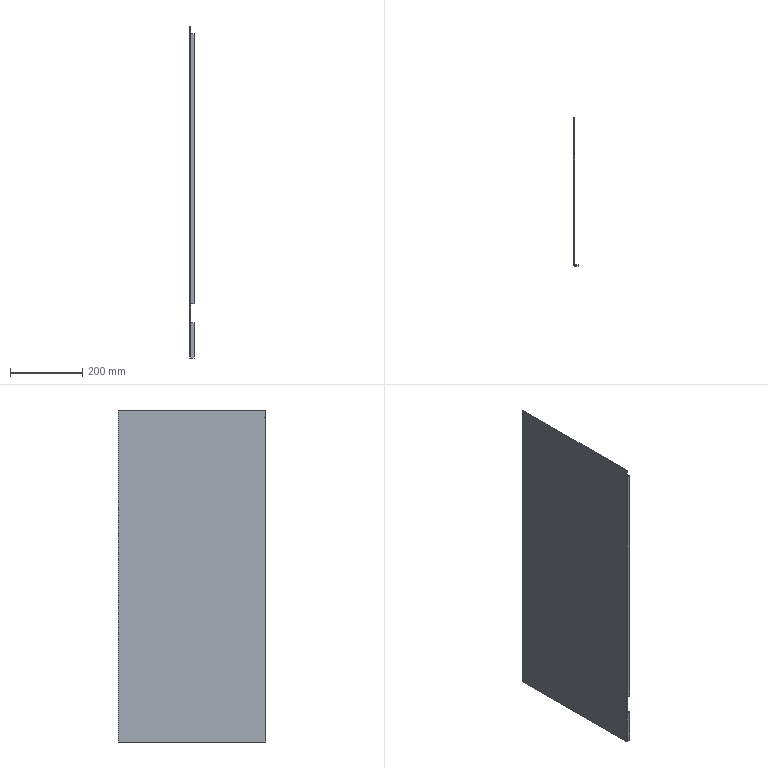Part | SolidWorks | 1 solid | 25 faces | box 12 x 410 x 920 mm | volume 770485 mm3 | plane 23 | cylinder 2 | commonest cylinder face diameters 0.2 x1 4.2 x1
STEP:
#1=CARTESIAN_POINT('',(10.,-205.,-460.));
#2=VERTEX_POINT('',#1);
#3=CARTESIAN_POINT('',(10.,-205.,-362.));
#4=VERTEX_POINT('',#3);
#5=CARTESIAN_POINT('',(10.,-205.,0.));
#6=DIRECTION('',(0.,0.,1.));
#7=VECTOR('',#6,1000.);
#8=LINE('',#5,#7);
#9=EDGE_CURVE('',#2,#4,#8,.T.);
#10=ORIENTED_EDGE('',*,*,#9,.T.);
#11=CARTESIAN_POINT('',(0.1,-205.,-362.));
#12=VERTEX_POINT('',#11);
#13=CARTESIAN_POINT('',(0.,-205.,-362.));
#14=DIRECTION('',(1.,0.,0.));
#15=VECTOR('',#14,1000.);
#16=LINE('',#13,#15);
#17=EDGE_CURVE('',#12,#4,#16,.T.);
#18=ORIENTED_EDGE('',*,*,#17,.F.);
#19=CARTESIAN_POINT('',(0.1,-205.,-460.));
#20=VERTEX_POINT('',#19);
#21=CARTESIAN_POINT('',(0.1,-205.,439.));
#22=DIRECTION('',(0.,0.,1.));
#23=VECTOR('',#22,1000.);
#24=LINE('',#21,#23);
#25=EDGE_CURVE('',#20,#12,#24,.T.);
#26=ORIENTED_EDGE('',*,*,#25,.F.);
#27=CARTESIAN_POINT('',(0.,-205.,-460.));
#28=DIRECTION('',(1.,0.,0.));
#29=VECTOR('',#28,1000.);
#30=LINE('',#27,#29);
#31=EDGE_CURVE('',#20,#2,#30,.T.);
#32=ORIENTED_EDGE('',*,*,#31,.T.);
#33=EDGE_LOOP('',(#10,#18,#26,#32));
#34=FACE_OUTER_BOUND('',#33,.T.);
#35=CARTESIAN_POINT('',(0.,-205.,0.));
#36=DIRECTION('',(0.,1.,0.));
#37=DIRECTION('',(-1.,0.,0.));
#38=AXIS2_PLACEMENT_3D('',#35,#36,#37);
#39=PLANE('',#38);
#40=ADVANCED_FACE('',(#34),#39,.F.);
#41=CARTESIAN_POINT('',(10.,-203.,-362.));
#42=VERTEX_POINT('',#41);
#43=CARTESIAN_POINT('',(0.1,-203.,-362.));
#44=VERTEX_POINT('',#43);
#45=CARTESIAN_POINT('',(0.,-203.,-362.));
#46=DIRECTION('',(-1.,0.,0.));
#47=VECTOR('',#46,1000.);
#48=LINE('',#45,#47);
#49=EDGE_CURVE('',#42,#44,#48,.T.);
#50=ORIENTED_EDGE('',*,*,#49,.F.);
#51=CARTESIAN_POINT('',(10.,-203.,-460.));
#52=VERTEX_POINT('',#51);
#53=CARTESIAN_POINT('',(10.,-203.,439.));
#54=DIRECTION('',(0.,0.,1.));
#55=VECTOR('',#54,1000.);
#56=LINE('',#53,#55);
#57=EDGE_CURVE('',#52,#42,#56,.T.);
#58=ORIENTED_EDGE('',*,*,#57,.F.);
#59=CARTESIAN_POINT('',(0.1,-203.,-460.));
#60=VERTEX_POINT('',#59);
#61=CARTESIAN_POINT('',(10.,-203.,-460.));
#62=DIRECTION('',(1.,0.,0.));
#63=VECTOR('',#62,1000.);
#64=LINE('',#61,#63);
#65=EDGE_CURVE('',#60,#52,#64,.T.);
#66=ORIENTED_EDGE('',*,*,#65,.F.);
#67=CARTESIAN_POINT('',(0.1,-203.,439.));
#68=DIRECTION('',(0.,0.,-1.));
#69=VECTOR('',#68,1000.);
#70=LINE('',#67,#69);
#71=EDGE_CURVE('',#44,#60,#70,.T.);
#72=ORIENTED_EDGE('',*,*,#71,.F.);
#73=EDGE_LOOP('',(#50,#58,#66,#72));
#74=FACE_OUTER_BOUND('',#73,.T.);
#75=CARTESIAN_POINT('',(0.,-203.,0.));
#76=DIRECTION('',(0.,1.,0.));
#77=DIRECTION('',(-1.,0.,0.));
#78=AXIS2_PLACEMENT_3D('',#75,#76,#77);
#79=PLANE('',#78);
#80=ADVANCED_FACE('',(#74),#79,.T.);
#81=ORIENTED_EDGE('',*,*,#57,.T.);
#82=CARTESIAN_POINT('',(10.,-205.001,-362.));
#83=DIRECTION('',(0.,1.,0.));
#84=VECTOR('',#83,1000.);
#85=LINE('',#82,#84);
#86=EDGE_CURVE('',#4,#42,#85,.T.);
#87=ORIENTED_EDGE('',*,*,#86,.F.);
#88=ORIENTED_EDGE('',*,*,#9,.F.);
#89=CARTESIAN_POINT('',(10.,-205.,-460.));
#90=DIRECTION('',(0.,1.,0.));
#91=VECTOR('',#90,1000.);
#92=LINE('',#89,#91);
#93=EDGE_CURVE('',#2,#52,#92,.T.);
#94=ORIENTED_EDGE('',*,*,#93,.T.);
#95=EDGE_LOOP('',(#81,#87,#88,#94));
#96=FACE_OUTER_BOUND('',#95,.T.);
#97=CARTESIAN_POINT('',(10.,-205.,439.));
#98=DIRECTION('',(-1.,0.,0.));
#99=DIRECTION('',(0.,-1.,0.));
#100=AXIS2_PLACEMENT_3D('',#97,#98,#99);
#101=PLANE('',#100);
#102=ADVANCED_FACE('',(#96),#101,.F.);
#103=CARTESIAN_POINT('',(0.,-202.9,-460.));
#104=VERTEX_POINT('',#103);
#105=CARTESIAN_POINT('',(0.,205.,-460.));
#106=VERTEX_POINT('',#105);
#107=CARTESIAN_POINT('',(0.,-205.,-460.));
#108=DIRECTION('',(0.,1.,0.));
#109=VECTOR('',#108,1000.);
#110=LINE('',#107,#109);
#111=EDGE_CURVE('',#104,#106,#110,.T.);
#112=ORIENTED_EDGE('',*,*,#111,.F.);
#113=CARTESIAN_POINT('',(-2.,-202.9,-460.));
#114=VERTEX_POINT('',#113);
#115=CARTESIAN_POINT('',(0.,-202.9,-460.));
#116=DIRECTION('',(-1.,0.,0.));
#117=VECTOR('',#116,1000.);
#118=LINE('',#115,#117);
#119=EDGE_CURVE('',#104,#114,#118,.T.);
#120=ORIENTED_EDGE('',*,*,#119,.T.);
#121=CARTESIAN_POINT('',(-2.,205.,-460.));
#122=VERTEX_POINT('',#121);
#123=CARTESIAN_POINT('',(-2.,-205.,-460.));
#124=DIRECTION('',(0.,1.,0.));
#125=VECTOR('',#124,1000.);
#126=LINE('',#123,#125);
#127=EDGE_CURVE('',#114,#122,#126,.T.);
#128=ORIENTED_EDGE('',*,*,#127,.T.);
#129=CARTESIAN_POINT('',(-2.,205.,-460.));
#130=DIRECTION('',(1.,0.,0.));
#131=VECTOR('',#130,1000.);
#132=LINE('',#129,#131);
#133=EDGE_CURVE('',#122,#106,#132,.T.);
#134=ORIENTED_EDGE('',*,*,#133,.T.);
#135=EDGE_LOOP('',(#112,#120,#128,#134));
#136=FACE_OUTER_BOUND('',#135,.T.);
#137=CARTESIAN_POINT('',(-2.,-205.,-460.));
#138=DIRECTION('',(0.,0.,-1.));
#139=DIRECTION('',(-1.,0.,0.));
#140=AXIS2_PLACEMENT_3D('',#137,#138,#139);
#141=PLANE('',#140);
#142=ADVANCED_FACE('',(#136),#141,.T.);
#143=CARTESIAN_POINT('',(-2.,-205.,460.));
#144=VERTEX_POINT('',#143);
#145=CARTESIAN_POINT('',(-2.,-205.,440.));
#146=VERTEX_POINT('',#145);
#147=CARTESIAN_POINT('',(-2.,-205.,-460.));
#148=DIRECTION('',(0.,0.,-1.));
#149=VECTOR('',#148,1000.);
#150=LINE('',#147,#149);
#151=EDGE_CURVE('',#144,#146,#150,.T.);
#152=ORIENTED_EDGE('',*,*,#151,.T.);
#153=CARTESIAN_POINT('',(0.,-205.,440.));
#154=VERTEX_POINT('',#153);
#155=CARTESIAN_POINT('',(0.,-205.,440.));
#156=DIRECTION('',(-1.,0.,0.));
#157=VECTOR('',#156,1000.);
#158=LINE('',#155,#157);
#159=EDGE_CURVE('',#154,#146,#158,.T.);
#160=ORIENTED_EDGE('',*,*,#159,.F.);
#161=CARTESIAN_POINT('',(0.,-205.,460.));
#162=VERTEX_POINT('',#161);
#163=CARTESIAN_POINT('',(0.,-205.,-460.));
#164=DIRECTION('',(0.,0.,-1.));
#165=VECTOR('',#164,1000.);
#166=LINE('',#163,#165);
#167=EDGE_CURVE('',#162,#154,#166,.T.);
#168=ORIENTED_EDGE('',*,*,#167,.F.);
#169=CARTESIAN_POINT('',(-2.,-205.,460.));
#170=DIRECTION('',(1.,0.,0.));
#171=VECTOR('',#170,1000.);
#172=LINE('',#169,#171);
#173=EDGE_CURVE('',#144,#162,#172,.T.);
#174=ORIENTED_EDGE('',*,*,#173,.F.);
#175=EDGE_LOOP('',(#152,#160,#168,#174));
#176=FACE_OUTER_BOUND('',#175,.T.);
#177=CARTESIAN_POINT('',(-2.,-205.,-460.));
#178=DIRECTION('',(0.,-1.,0.));
#179=DIRECTION('',(0.,0.,-1.));
#180=AXIS2_PLACEMENT_3D('',#177,#178,#179);
#181=PLANE('',#180);
#182=ADVANCED_FACE('',(#176),#181,.T.);
#183=CARTESIAN_POINT('',(-2.,-202.9,439.));
#184=VERTEX_POINT('',#183);
#185=CARTESIAN_POINT('',(-2.,-202.9,-460.));
#186=DIRECTION('',(0.,0.,1.));
#187=VECTOR('',#186,1000.);
#188=LINE('',#185,#187);
#189=EDGE_CURVE('',#114,#184,#188,.T.);
#190=ORIENTED_EDGE('',*,*,#189,.T.);
#191=CARTESIAN_POINT('',(-2.,-201.9,439.));
#192=VERTEX_POINT('',#191);
#193=CARTESIAN_POINT('',(-2.,0.,439.));
#194=DIRECTION('',(0.,-1.,0.));
#195=VECTOR('',#194,1000.);
#196=LINE('',#193,#195);
#197=EDGE_CURVE('',#192,#184,#196,.T.);
#198=ORIENTED_EDGE('',*,*,#197,.F.);
#199=CARTESIAN_POINT('',(-2.,-201.9,440.));
#200=VERTEX_POINT('',#199);
#201=CARTESIAN_POINT('',(-2.,-201.9,0.));
#202=DIRECTION('',(0.,0.,-1.));
#203=VECTOR('',#202,1000.);
#204=LINE('',#201,#203);
#205=EDGE_CURVE('',#200,#192,#204,.T.);
#206=ORIENTED_EDGE('',*,*,#205,.F.);
#207=CARTESIAN_POINT('',(-2.,0.,440.));
#208=DIRECTION('',(0.,1.,0.));
#209=VECTOR('',#208,1000.);
#210=LINE('',#207,#209);
#211=EDGE_CURVE('',#146,#200,#210,.T.);
#212=ORIENTED_EDGE('',*,*,#211,.F.);
#213=ORIENTED_EDGE('',*,*,#151,.F.);
#214=CARTESIAN_POINT('',(-2.,205.,460.));
#215=VERTEX_POINT('',#214);
#216=CARTESIAN_POINT('',(-2.,-205.,460.));
#217=DIRECTION('',(0.,-1.,0.));
#218=VECTOR('',#217,1000.);
#219=LINE('',#216,#218);
#220=EDGE_CURVE('',#215,#144,#219,.T.);
#221=ORIENTED_EDGE('',*,*,#220,.F.);
#222=CARTESIAN_POINT('',(-2.,205.,-460.));
#223=DIRECTION('',(0.,0.,1.));
#224=VECTOR('',#223,1000.);
#225=LINE('',#222,#224);
#226=EDGE_CURVE('',#122,#215,#225,.T.);
#227=ORIENTED_EDGE('',*,*,#226,.F.);
#228=ORIENTED_EDGE('',*,*,#127,.F.);
#229=EDGE_LOOP('',(#190,#198,#206,#212,#213,#221,#227,#228));
#230=FACE_OUTER_BOUND('',#229,.T.);
#231=CARTESIAN_POINT('',(-2.,0.,0.));
#232=DIRECTION('',(1.,0.,0.));
#233=DIRECTION('',(0.,0.,-1.));
#234=AXIS2_PLACEMENT_3D('',#231,#232,#233);
#235=PLANE('',#234);
#236=ADVANCED_FACE('',(#230),#235,.F.);
#237=CARTESIAN_POINT('',(0.,-202.9,439.));
#238=VERTEX_POINT('',#237);
#239=CARTESIAN_POINT('',(0.,-201.9,439.));
#240=VERTEX_POINT('',#239);
#241=CARTESIAN_POINT('',(0.,-202.9,439.));
#242=DIRECTION('',(0.,1.,0.));
#243=VECTOR('',#242,1000.);
#244=LINE('',#241,#243);
#245=EDGE_CURVE('',#238,#240,#244,.T.);
#246=ORIENTED_EDGE('',*,*,#245,.F.);
#247=CARTESIAN_POINT('',(0.,-202.9,-460.));
#248=DIRECTION('',(0.,0.,1.));
#249=VECTOR('',#248,1000.);
#250=LINE('',#247,#249);
#251=EDGE_CURVE('',#104,#238,#250,.T.);
#252=ORIENTED_EDGE('',*,*,#251,.F.);
#253=ORIENTED_EDGE('',*,*,#111,.T.);
#254=CARTESIAN_POINT('',(0.,205.,460.));
#255=VERTEX_POINT('',#254);
#256=CARTESIAN_POINT('',(0.,205.,-460.));
#257=DIRECTION('',(0.,0.,1.));
#258=VECTOR('',#257,1000.);
#259=LINE('',#256,#258);
#260=EDGE_CURVE('',#106,#255,#259,.T.);
#261=ORIENTED_EDGE('',*,*,#260,.T.);
#262=CARTESIAN_POINT('',(0.,-205.,460.));
#263=DIRECTION('',(0.,-1.,0.));
#264=VECTOR('',#263,1000.);
#265=LINE('',#262,#264);
#266=EDGE_CURVE('',#255,#162,#265,.T.);
#267=ORIENTED_EDGE('',*,*,#266,.T.);
#268=ORIENTED_EDGE('',*,*,#167,.T.);
#269=CARTESIAN_POINT('',(0.,-201.9,440.));
#270=VERTEX_POINT('',#269);
#271=CARTESIAN_POINT('',(0.,-201.9,440.));
#272=DIRECTION('',(0.,-1.,0.));
#273=VECTOR('',#272,1000.);
#274=LINE('',#271,#273);
#275=EDGE_CURVE('',#270,#154,#274,.T.);
#276=ORIENTED_EDGE('',*,*,#275,.F.);
#277=CARTESIAN_POINT('',(0.,-201.9,439.));
#278=DIRECTION('',(0.,0.,1.));
#279=VECTOR('',#278,1000.);
#280=LINE('',#277,#279);
#281=EDGE_CURVE('',#240,#270,#280,.T.);
#282=ORIENTED_EDGE('',*,*,#281,.F.);
#283=EDGE_LOOP('',(#246,#252,#253,#261,#267,#268,#276,#282));
#284=FACE_OUTER_BOUND('',#283,.T.);
#285=CARTESIAN_POINT('',(0.,0.,0.));
#286=DIRECTION('',(1.,0.,0.));
#287=DIRECTION('',(0.,0.,-1.));
#288=AXIS2_PLACEMENT_3D('',#285,#286,#287);
#289=PLANE('',#288);
#290=ADVANCED_FACE('',(#284),#289,.T.);
#291=ORIENTED_EDGE('',*,*,#266,.F.);
#292=CARTESIAN_POINT('',(-2.,205.,460.));
#293=DIRECTION('',(1.,0.,0.));
#294=VECTOR('',#293,1000.);
#295=LINE('',#292,#294);
#296=EDGE_CURVE('',#215,#255,#295,.T.);
#297=ORIENTED_EDGE('',*,*,#296,.F.);
#298=ORIENTED_EDGE('',*,*,#220,.T.);
#299=ORIENTED_EDGE('',*,*,#173,.T.);
#300=EDGE_LOOP('',(#291,#297,#298,#299));
#301=FACE_OUTER_BOUND('',#300,.T.);
#302=CARTESIAN_POINT('',(-2.,-205.,460.));
#303=DIRECTION('',(0.,0.,1.));
#304=DIRECTION('',(1.,0.,0.));
#305=AXIS2_PLACEMENT_3D('',#302,#303,#304);
#306=PLANE('',#305);
#307=ADVANCED_FACE('',(#301),#306,.T.);
#308=ORIENTED_EDGE('',*,*,#260,.F.);
#309=ORIENTED_EDGE('',*,*,#133,.F.);
#310=ORIENTED_EDGE('',*,*,#226,.T.);
#311=ORIENTED_EDGE('',*,*,#296,.T.);
#312=EDGE_LOOP('',(#308,#309,#310,#311));
#313=FACE_OUTER_BOUND('',#312,.T.);
#314=CARTESIAN_POINT('',(-2.,205.,-460.));
#315=DIRECTION('',(0.,1.,0.));
#316=DIRECTION('',(0.,0.,1.));
#317=AXIS2_PLACEMENT_3D('',#314,#315,#316);
#318=PLANE('',#317);
#319=ADVANCED_FACE('',(#313),#318,.T.);
#320=CARTESIAN_POINT('',(0.,-201.9,439.));
#321=DIRECTION('',(-1.,0.,0.));
#322=VECTOR('',#321,1000.);
#323=LINE('',#320,#322);
#324=EDGE_CURVE('',#240,#192,#323,.T.);
#325=ORIENTED_EDGE('',*,*,#324,.T.);
#326=ORIENTED_EDGE('',*,*,#197,.T.);
#327=CARTESIAN_POINT('',(0.,-202.9,439.));
#328=DIRECTION('',(-1.,0.,0.));
#329=VECTOR('',#328,1000.);
#330=LINE('',#327,#329);
#331=EDGE_CURVE('',#238,#184,#330,.T.);
#332=ORIENTED_EDGE('',*,*,#331,.F.);
#333=ORIENTED_EDGE('',*,*,#245,.T.);
#334=EDGE_LOOP('',(#325,#326,#332,#333));
#335=FACE_OUTER_BOUND('',#334,.T.);
#336=CARTESIAN_POINT('',(0.,-202.9,439.));
#337=DIRECTION('',(0.,0.,1.));
#338=DIRECTION('',(1.,0.,0.));
#339=AXIS2_PLACEMENT_3D('',#336,#337,#338);
#340=PLANE('',#339);
#341=ADVANCED_FACE('',(#335),#340,.T.);
#342=CARTESIAN_POINT('',(0.,-201.9,440.));
#343=DIRECTION('',(-1.,0.,0.));
#344=VECTOR('',#343,1000.);
#345=LINE('',#342,#344);
#346=EDGE_CURVE('',#270,#200,#345,.T.);
#347=ORIENTED_EDGE('',*,*,#346,.T.);
#348=ORIENTED_EDGE('',*,*,#205,.T.);
#349=ORIENTED_EDGE('',*,*,#324,.F.);
#350=ORIENTED_EDGE('',*,*,#281,.T.);
#351=EDGE_LOOP('',(#347,#348,#349,#350));
#352=FACE_OUTER_BOUND('',#351,.T.);
#353=CARTESIAN_POINT('',(0.,-201.9,439.));
#354=DIRECTION('',(0.,-1.,0.));
#355=DIRECTION('',(0.,0.,-1.));
#356=AXIS2_PLACEMENT_3D('',#353,#354,#355);
#357=PLANE('',#356);
#358=ADVANCED_FACE('',(#352),#357,.T.);
#359=ORIENTED_EDGE('',*,*,#159,.T.);
#360=ORIENTED_EDGE('',*,*,#211,.T.);
#361=ORIENTED_EDGE('',*,*,#346,.F.);
#362=ORIENTED_EDGE('',*,*,#275,.T.);
#363=EDGE_LOOP('',(#359,#360,#361,#362));
#364=FACE_OUTER_BOUND('',#363,.T.);
#365=CARTESIAN_POINT('',(0.,-201.9,440.));
#366=DIRECTION('',(0.,0.,-1.));
#367=DIRECTION('',(-1.,0.,0.));
#368=AXIS2_PLACEMENT_3D('',#365,#366,#367);
#369=PLANE('',#368);
#370=ADVANCED_FACE('',(#364),#369,.T.);
#371=CARTESIAN_POINT('',(0.1,-203.,439.));
#372=VERTEX_POINT('',#371);
#373=CARTESIAN_POINT('',(0.1,-205.,439.));
#374=VERTEX_POINT('',#373);
#375=CARTESIAN_POINT('',(0.1,-205.,439.));
#376=DIRECTION('',(0.,-1.,0.));
#377=VECTOR('',#376,1000.);
#378=LINE('',#375,#377);
#379=EDGE_CURVE('',#372,#374,#378,.T.);
#380=ORIENTED_EDGE('',*,*,#379,.F.);
#381=CARTESIAN_POINT('',(0.1,-202.9,439.));
#382=DIRECTION('',(0.,0.,1.));
#383=DIRECTION('',(-1.,0.,0.));
#384=AXIS2_PLACEMENT_3D('',#381,#382,#383);
#385=CIRCLE('',#384,0.1);
#386=EDGE_CURVE('',#238,#372,#385,.T.);
#387=ORIENTED_EDGE('',*,*,#386,.F.);
#388=ORIENTED_EDGE('',*,*,#331,.T.);
#389=CARTESIAN_POINT('',(0.1,-202.9,439.));
#390=DIRECTION('',(0.,0.,1.));
#391=DIRECTION('',(-1.,0.,0.));
#392=AXIS2_PLACEMENT_3D('',#389,#390,#391);
#393=CIRCLE('',#392,2.1);
#394=EDGE_CURVE('',#184,#374,#393,.T.);
#395=ORIENTED_EDGE('',*,*,#394,.T.);
#396=EDGE_LOOP('',(#380,#387,#388,#395));
#397=FACE_OUTER_BOUND('',#396,.T.);
#398=CARTESIAN_POINT('',(0.1,-202.9,439.));
#399=DIRECTION('',(0.,0.,1.));
#400=DIRECTION('',(1.,0.,0.));
#401=AXIS2_PLACEMENT_3D('',#398,#399,#400);
#402=PLANE('',#401);
#403=ADVANCED_FACE('',(#397),#402,.T.);
#404=CARTESIAN_POINT('',(0.1,-202.9,-460.));
#405=DIRECTION('',(0.,0.,-1.));
#406=DIRECTION('',(-1.,0.,0.));
#407=AXIS2_PLACEMENT_3D('',#404,#405,#406);
#408=CIRCLE('',#407,0.1);
#409=EDGE_CURVE('',#60,#104,#408,.T.);
#410=ORIENTED_EDGE('',*,*,#409,.F.);
#411=CARTESIAN_POINT('',(0.1,-203.,-460.));
#412=DIRECTION('',(0.,-1.,0.));
#413=VECTOR('',#412,1000.);
#414=LINE('',#411,#413);
#415=EDGE_CURVE('',#60,#20,#414,.T.);
#416=ORIENTED_EDGE('',*,*,#415,.T.);
#417=CARTESIAN_POINT('',(0.1,-202.9,-460.));
#418=DIRECTION('',(0.,0.,-1.));
#419=DIRECTION('',(-1.,0.,0.));
#420=AXIS2_PLACEMENT_3D('',#417,#418,#419);
#421=CIRCLE('',#420,2.1);
#422=EDGE_CURVE('',#20,#114,#421,.T.);
#423=ORIENTED_EDGE('',*,*,#422,.T.);
#424=ORIENTED_EDGE('',*,*,#119,.F.);
#425=EDGE_LOOP('',(#410,#416,#423,#424));
#426=FACE_OUTER_BOUND('',#425,.T.);
#427=CARTESIAN_POINT('',(0.1,-202.9,-460.));
#428=DIRECTION('',(0.,0.,1.));
#429=DIRECTION('',(1.,0.,0.));
#430=AXIS2_PLACEMENT_3D('',#427,#428,#429);
#431=PLANE('',#430);
#432=ADVANCED_FACE('',(#426),#431,.F.);
#433=CARTESIAN_POINT('',(0.,-204.998,-362.));
#434=VERTEX_POINT('',#433);
#435=CARTESIAN_POINT('',(0.1,-202.9,-362.));
#436=DIRECTION('',(0.,0.,-1.));
#437=DIRECTION('',(0.,1.,0.));
#438=AXIS2_PLACEMENT_3D('',#435,#436,#437);
#439=CIRCLE('',#438,2.1);
#440=EDGE_CURVE('',#12,#434,#439,.T.);
#441=ORIENTED_EDGE('',*,*,#440,.T.);
#442=CARTESIAN_POINT('',(0.,-204.998,-310.));
#443=VERTEX_POINT('',#442);
#444=CARTESIAN_POINT('',(0.,-204.998,-460.));
#445=DIRECTION('',(0.,0.,1.));
#446=VECTOR('',#445,1000.);
#447=LINE('',#444,#446);
#448=EDGE_CURVE('',#434,#443,#447,.T.);
#449=ORIENTED_EDGE('',*,*,#448,.T.);
#450=CARTESIAN_POINT('',(0.1,-205.,-310.));
#451=VERTEX_POINT('',#450);
#452=CARTESIAN_POINT('',(0.1,-202.9,-310.));
#453=DIRECTION('',(0.,0.,1.));
#454=DIRECTION('',(0.,-1.,0.));
#455=AXIS2_PLACEMENT_3D('',#452,#453,#454);
#456=CIRCLE('',#455,2.1);
#457=EDGE_CURVE('',#443,#451,#456,.T.);
#458=ORIENTED_EDGE('',*,*,#457,.T.);
#459=CARTESIAN_POINT('',(0.1,-205.,439.));
#460=DIRECTION('',(0.,0.,1.));
#461=VECTOR('',#460,1000.);
#462=LINE('',#459,#461);
#463=EDGE_CURVE('',#451,#374,#462,.T.);
#464=ORIENTED_EDGE('',*,*,#463,.T.);
#465=ORIENTED_EDGE('',*,*,#394,.F.);
#466=ORIENTED_EDGE('',*,*,#189,.F.);
#467=ORIENTED_EDGE('',*,*,#422,.F.);
#468=ORIENTED_EDGE('',*,*,#25,.T.);
#469=EDGE_LOOP('',(#441,#449,#458,#464,#465,#466,#467,#468));
#470=FACE_OUTER_BOUND('',#469,.T.);
#471=CARTESIAN_POINT('',(0.1,-202.9,-460.));
#472=DIRECTION('',(0.,0.,-1.));
#473=DIRECTION('',(0.,-1.,0.));
#474=AXIS2_PLACEMENT_3D('',#471,#472,#473);
#475=CYLINDRICAL_SURFACE('',#474,2.1);
#476=ADVANCED_FACE('',(#470),#475,.T.);
#477=ORIENTED_EDGE('',*,*,#251,.T.);
#478=ORIENTED_EDGE('',*,*,#386,.T.);
#479=CARTESIAN_POINT('',(0.1,-203.,-310.));
#480=VERTEX_POINT('',#479);
#481=CARTESIAN_POINT('',(0.1,-203.,439.));
#482=DIRECTION('',(0.,0.,-1.));
#483=VECTOR('',#482,1000.);
#484=LINE('',#481,#483);
#485=EDGE_CURVE('',#372,#480,#484,.T.);
#486=ORIENTED_EDGE('',*,*,#485,.T.);
#487=CARTESIAN_POINT('',(0.1,-203.,-460.));
#488=DIRECTION('',(0.,0.,1.));
#489=VECTOR('',#488,1000.);
#490=LINE('',#487,#489);
#491=EDGE_CURVE('',#44,#480,#490,.T.);
#492=ORIENTED_EDGE('',*,*,#491,.F.);
#493=ORIENTED_EDGE('',*,*,#71,.T.);
#494=ORIENTED_EDGE('',*,*,#409,.T.);
#495=EDGE_LOOP('',(#477,#478,#486,#492,#493,#494));
#496=FACE_OUTER_BOUND('',#495,.T.);
#497=CARTESIAN_POINT('',(0.1,-202.9,-460.));
#498=DIRECTION('',(0.,0.,-1.));
#499=DIRECTION('',(0.,-1.,0.));
#500=AXIS2_PLACEMENT_3D('',#497,#498,#499);
#501=CYLINDRICAL_SURFACE('',#500,0.1);
#502=ADVANCED_FACE('',(#496),#501,.F.);
#503=ORIENTED_EDGE('',*,*,#415,.F.);
#504=ORIENTED_EDGE('',*,*,#65,.T.);
#505=ORIENTED_EDGE('',*,*,#93,.F.);
#506=ORIENTED_EDGE('',*,*,#31,.F.);
#507=EDGE_LOOP('',(#503,#504,#505,#506));
#508=FACE_OUTER_BOUND('',#507,.T.);
#509=CARTESIAN_POINT('',(10.,-205.,-460.));
#510=DIRECTION('',(0.,0.,1.));
#511=DIRECTION('',(0.,-1.,0.));
#512=AXIS2_PLACEMENT_3D('',#509,#510,#511);
#513=PLANE('',#512);
#514=ADVANCED_FACE('',(#508),#513,.F.);
#515=ORIENTED_EDGE('',*,*,#379,.T.);
#516=CARTESIAN_POINT('',(10.,-205.,439.));
#517=VERTEX_POINT('',#516);
#518=CARTESIAN_POINT('',(0.,-205.,439.));
#519=DIRECTION('',(-1.,0.,0.));
#520=VECTOR('',#519,1000.);
#521=LINE('',#518,#520);
#522=EDGE_CURVE('',#517,#374,#521,.T.);
#523=ORIENTED_EDGE('',*,*,#522,.F.);
#524=CARTESIAN_POINT('',(10.,-203.,439.));
#525=VERTEX_POINT('',#524);
#526=CARTESIAN_POINT('',(10.,-205.,439.));
#527=DIRECTION('',(0.,1.,0.));
#528=VECTOR('',#527,1000.);
#529=LINE('',#526,#528);
#530=EDGE_CURVE('',#517,#525,#529,.T.);
#531=ORIENTED_EDGE('',*,*,#530,.T.);
#532=CARTESIAN_POINT('',(0.,-203.,439.));
#533=DIRECTION('',(-1.,0.,0.));
#534=VECTOR('',#533,1000.);
#535=LINE('',#532,#534);
#536=EDGE_CURVE('',#525,#372,#535,.T.);
#537=ORIENTED_EDGE('',*,*,#536,.T.);
#538=EDGE_LOOP('',(#515,#523,#531,#537));
#539=FACE_OUTER_BOUND('',#538,.T.);
#540=CARTESIAN_POINT('',(0.,-205.,439.));
#541=DIRECTION('',(0.,0.,-1.));
#542=DIRECTION('',(0.,1.,0.));
#543=AXIS2_PLACEMENT_3D('',#540,#541,#542);
#544=PLANE('',#543);
#545=ADVANCED_FACE('',(#539),#544,.F.);
#546=ORIENTED_EDGE('',*,*,#463,.F.);
#547=CARTESIAN_POINT('',(10.,-205.,-310.));
#548=VERTEX_POINT('',#547);
#549=CARTESIAN_POINT('',(0.,-205.,-310.));
#550=DIRECTION('',(-1.,0.,0.));
#551=VECTOR('',#550,1000.);
#552=LINE('',#549,#551);
#553=EDGE_CURVE('',#548,#451,#552,.T.);
#554=ORIENTED_EDGE('',*,*,#553,.F.);
#555=CARTESIAN_POINT('',(10.,-205.,0.));
#556=DIRECTION('',(0.,0.,1.));
#557=VECTOR('',#556,1000.);
#558=LINE('',#555,#557);
#559=EDGE_CURVE('',#548,#517,#558,.T.);
#560=ORIENTED_EDGE('',*,*,#559,.T.);
#561=ORIENTED_EDGE('',*,*,#522,.T.);
#562=EDGE_LOOP('',(#546,#554,#560,#561));
#563=FACE_OUTER_BOUND('',#562,.T.);
#564=CARTESIAN_POINT('',(0.,-205.,0.));
#565=DIRECTION('',(0.,1.,0.));
#566=DIRECTION('',(-1.,0.,0.));
#567=AXIS2_PLACEMENT_3D('',#564,#565,#566);
#568=PLANE('',#567);
#569=ADVANCED_FACE('',(#563),#568,.F.);
#570=CARTESIAN_POINT('',(10.,-203.,-310.));
#571=VERTEX_POINT('',#570);
#572=CARTESIAN_POINT('',(0.,-203.,-310.));
#573=DIRECTION('',(1.,0.,0.));
#574=VECTOR('',#573,1000.);
#575=LINE('',#572,#574);
#576=EDGE_CURVE('',#480,#571,#575,.T.);
#577=ORIENTED_EDGE('',*,*,#576,.F.);
#578=ORIENTED_EDGE('',*,*,#485,.F.);
#579=ORIENTED_EDGE('',*,*,#536,.F.);
#580=CARTESIAN_POINT('',(10.,-203.,439.));
#581=DIRECTION('',(0.,0.,1.));
#582=VECTOR('',#581,1000.);
#583=LINE('',#580,#582);
#584=EDGE_CURVE('',#571,#525,#583,.T.);
#585=ORIENTED_EDGE('',*,*,#584,.F.);
#586=EDGE_LOOP('',(#577,#578,#579,#585));
#587=FACE_OUTER_BOUND('',#586,.T.);
#588=CARTESIAN_POINT('',(0.,-203.,0.));
#589=DIRECTION('',(0.,1.,0.));
#590=DIRECTION('',(-1.,0.,0.));
#591=AXIS2_PLACEMENT_3D('',#588,#589,#590);
#592=PLANE('',#591);
#593=ADVANCED_FACE('',(#587),#592,.T.);
#594=ORIENTED_EDGE('',*,*,#559,.F.);
#595=CARTESIAN_POINT('',(10.,-205.001,-310.));
#596=DIRECTION('',(0.,-1.,0.));
#597=VECTOR('',#596,1000.);
#598=LINE('',#595,#597);
#599=EDGE_CURVE('',#571,#548,#598,.T.);
#600=ORIENTED_EDGE('',*,*,#599,.F.);
#601=ORIENTED_EDGE('',*,*,#584,.T.);
#602=ORIENTED_EDGE('',*,*,#530,.F.);
#603=EDGE_LOOP('',(#594,#600,#601,#602));
#604=FACE_OUTER_BOUND('',#603,.T.);
#605=CARTESIAN_POINT('',(10.,-205.,439.));
#606=DIRECTION('',(-1.,0.,0.));
#607=DIRECTION('',(0.,-1.,0.));
#608=AXIS2_PLACEMENT_3D('',#605,#606,#607);
#609=PLANE('',#608);
#610=ADVANCED_FACE('',(#604),#609,.F.);
#611=ORIENTED_EDGE('',*,*,#491,.T.);
#612=CARTESIAN_POINT('',(0.,-203.,-310.));
#613=VERTEX_POINT('',#612);
#614=CARTESIAN_POINT('',(0.,-203.,-310.));
#615=DIRECTION('',(1.,0.,0.));
#616=VECTOR('',#615,1000.);
#617=LINE('',#614,#616);
#618=EDGE_CURVE('',#613,#480,#617,.T.);
#619=ORIENTED_EDGE('',*,*,#618,.F.);
#620=CARTESIAN_POINT('',(0.,-203.,-362.));
#621=VERTEX_POINT('',#620);
#622=CARTESIAN_POINT('',(0.,-203.,-362.));
#623=DIRECTION('',(0.,0.,1.));
#624=VECTOR('',#623,1000.);
#625=LINE('',#622,#624);
#626=EDGE_CURVE('',#621,#613,#625,.T.);
#627=ORIENTED_EDGE('',*,*,#626,.F.);
#628=CARTESIAN_POINT('',(0.,-203.,-362.));
#629=DIRECTION('',(-1.,0.,0.));
#630=VECTOR('',#629,1000.);
#631=LINE('',#628,#630);
#632=EDGE_CURVE('',#44,#621,#631,.T.);
#633=ORIENTED_EDGE('',*,*,#632,.F.);
#634=EDGE_LOOP('',(#611,#619,#627,#633));
#635=FACE_OUTER_BOUND('',#634,.T.);
#636=CARTESIAN_POINT('',(0.,-203.,0.));
#637=DIRECTION('',(0.,1.,0.));
#638=DIRECTION('',(-1.,0.,0.));
#639=AXIS2_PLACEMENT_3D('',#636,#637,#638);
#640=PLANE('',#639);
#641=ADVANCED_FACE('',(#635),#640,.F.);
#642=CARTESIAN_POINT('',(0.,-205.001,-362.));
#643=DIRECTION('',(0.,1.,0.));
#644=VECTOR('',#643,1000.);
#645=LINE('',#642,#644);
#646=EDGE_CURVE('',#434,#621,#645,.T.);
#647=ORIENTED_EDGE('',*,*,#646,.T.);
#648=ORIENTED_EDGE('',*,*,#626,.T.);
#649=CARTESIAN_POINT('',(0.,-205.001,-310.));
#650=DIRECTION('',(0.,1.,0.));
#651=VECTOR('',#650,1000.);
#652=LINE('',#649,#651);
#653=EDGE_CURVE('',#443,#613,#652,.T.);
#654=ORIENTED_EDGE('',*,*,#653,.F.);
#655=ORIENTED_EDGE('',*,*,#448,.F.);
#656=EDGE_LOOP('',(#647,#648,#654,#655));
#657=FACE_OUTER_BOUND('',#656,.T.);
#658=CARTESIAN_POINT('',(0.,-205.001,-362.));
#659=DIRECTION('',(-1.,0.,0.));
#660=DIRECTION('',(0.,-1.,0.));
#661=AXIS2_PLACEMENT_3D('',#658,#659,#660);
#662=PLANE('',#661);
#663=ADVANCED_FACE('',(#657),#662,.F.);
#664=ORIENTED_EDGE('',*,*,#17,.T.);
#665=ORIENTED_EDGE('',*,*,#86,.T.);
#666=ORIENTED_EDGE('',*,*,#49,.T.);
#667=ORIENTED_EDGE('',*,*,#632,.T.);
#668=ORIENTED_EDGE('',*,*,#646,.F.);
#669=ORIENTED_EDGE('',*,*,#440,.F.);
#670=EDGE_LOOP('',(#664,#665,#666,#667,#668,#669));
#671=FACE_OUTER_BOUND('',#670,.T.);
#672=CARTESIAN_POINT('',(0.,-205.001,-362.));
#673=DIRECTION('',(0.,0.,-1.));
#674=DIRECTION('',(0.,1.,0.));
#675=AXIS2_PLACEMENT_3D('',#672,#673,#674);
#676=PLANE('',#675);
#677=ADVANCED_FACE('',(#671),#676,.F.);
#678=ORIENTED_EDGE('',*,*,#653,.T.);
#679=ORIENTED_EDGE('',*,*,#618,.T.);
#680=ORIENTED_EDGE('',*,*,#576,.T.);
#681=ORIENTED_EDGE('',*,*,#599,.T.);
#682=ORIENTED_EDGE('',*,*,#553,.T.);
#683=ORIENTED_EDGE('',*,*,#457,.F.);
#684=EDGE_LOOP('',(#678,#679,#680,#681,#682,#683));
#685=FACE_OUTER_BOUND('',#684,.T.);
#686=CARTESIAN_POINT('',(0.,-205.001,-310.));
#687=DIRECTION('',(0.,0.,1.));
#688=DIRECTION('',(0.,-1.,0.));
#689=AXIS2_PLACEMENT_3D('',#686,#687,#688);
#690=PLANE('',#689);
#691=ADVANCED_FACE('',(#685),#690,.F.);
#692=CLOSED_SHELL('',(#40,#80,#102,#142,#182,#236,#290,#307,#319,#341,#358,#370,#403,#432,#476,#502,#514,#545,#569,#593,#610,#641,#663,#677,#691));
#693=MANIFOLD_SOLID_BREP('',#692);
#694=CARTESIAN_POINT('',(0.,0.,0.));
#695=DIRECTION('',(0.,0.,1.));
#696=DIRECTION('',(1.,0.,0.));
#697=AXIS2_PLACEMENT_3D('',#694,#695,#696);
#698=(LENGTH_UNIT()NAMED_UNIT(*)SI_UNIT(.MILLI.,.METRE.));
#699=UNCERTAINTY_MEASURE_WITH_UNIT(LENGTH_MEASURE(0.00001),#698,'','');
#700=(NAMED_UNIT(*)PLANE_ANGLE_UNIT()SI_UNIT($,.RADIAN.));
#701=(NAMED_UNIT(*)SI_UNIT($,.STERADIAN.)SOLID_ANGLE_UNIT());
#702=(GEOMETRIC_REPRESENTATION_CONTEXT(3)GLOBAL_UNCERTAINTY_ASSIGNED_CONTEXT((#699))GLOBAL_UNIT_ASSIGNED_CONTEXT((#698,#700,#701))REPRESENTATION_CONTEXT('',''));
#703=ADVANCED_BREP_SHAPE_REPRESENTATION('',(#693,#697),#702);